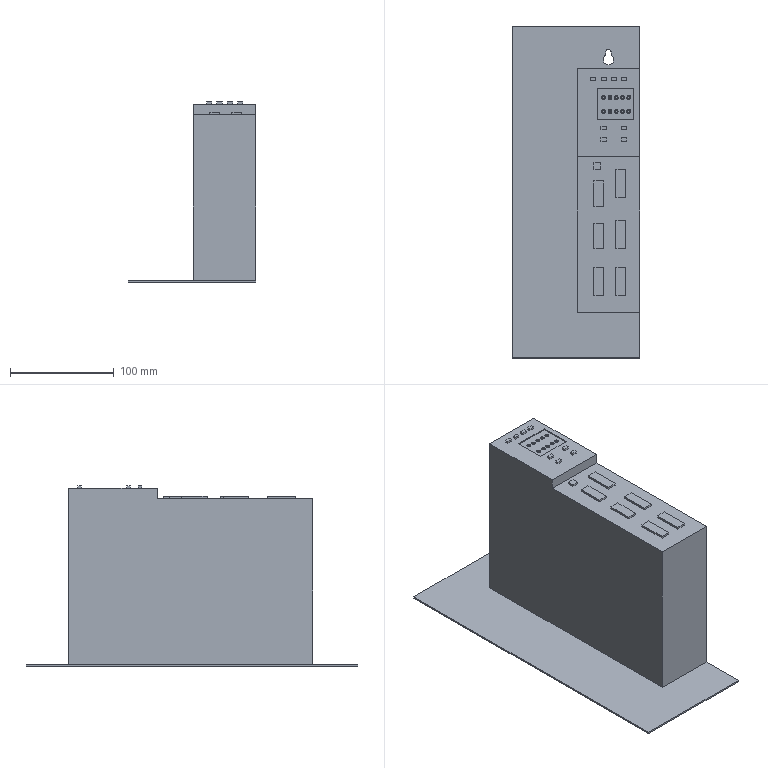Part | STEP file | f401kongzhiqi | 1 solid | 218 faces | box 122.5 x 320 x 173.5 mm | volume 2367856 mm3 | plane 114 | spline 100 | cylinder 4 | commonest cylinder face diameters 10 x3 5 x1